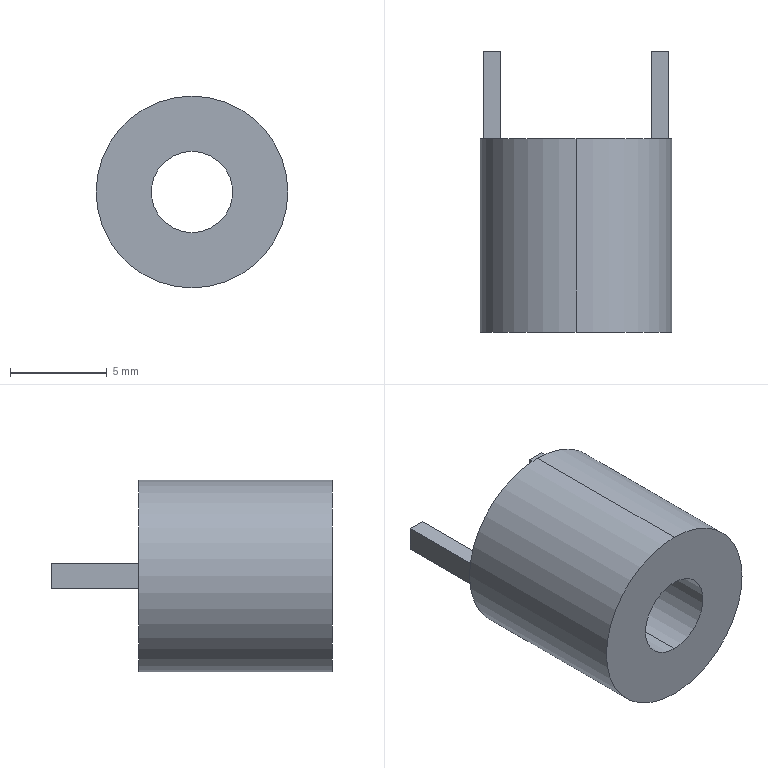Part | STEP file | 1 solid | 16 faces | box 9.9 x 14.5 x 9.9 mm | volume 641.755 mm3 | plane 12 | cylinder 4 | commonest cylinder face diameters 4.2 x2 9.9 x2
STEP:
#1=CARTESIAN_POINT('',(0.,0.,0.));
#2=DIRECTION('',(0.,0.,1.));
#3=DIRECTION('',(1.,0.,0.));
#4=AXIS2_PLACEMENT_3D('',#1,#2,#3);
#5=CARTESIAN_POINT('',(0.,0.,2.1));
#6=VERTEX_POINT('',#5);
#7=CARTESIAN_POINT('',(0.,10.,2.1));
#8=VERTEX_POINT('',#7);
#9=CARTESIAN_POINT('',(0.,10.,2.1));
#10=DIRECTION('',(0.,1.,0.));
#11=VECTOR('',#10,1.);
#12=LINE('',#9,#11);
#13=CARTESIAN_POINT('',(0.,10.,0.));
#14=DIRECTION('',(0.,1.,0.));
#15=DIRECTION('',(0.,0.,1.));
#16=AXIS2_PLACEMENT_3D('',#13,#14,#15);
#17=CYLINDRICAL_SURFACE('',#16,2.1);
#18=CARTESIAN_POINT('',(6.283,0.));
#19=DIRECTION('',(0.,1.));
#20=VECTOR('',#19,1.);
#21=LINE('',#18,#20);
#22=(GEOMETRIC_REPRESENTATION_CONTEXT(2)PARAMETRIC_REPRESENTATION_CONTEXT()REPRESENTATION_CONTEXT('',''));
#23=DEFINITIONAL_REPRESENTATION('',(#21),#22);
#24=PCURVE('',#17,#23);
#25=CARTESIAN_POINT('',(0.,10.,0.));
#26=DIRECTION('',(0.,1.,0.));
#27=DIRECTION('',(0.,0.,1.));
#28=AXIS2_PLACEMENT_3D('',#25,#26,#27);
#29=CYLINDRICAL_SURFACE('',#28,2.1);
#30=CARTESIAN_POINT('',(0.,0.));
#31=DIRECTION('',(0.,1.));
#32=VECTOR('',#31,1.);
#33=LINE('',#30,#32);
#34=(GEOMETRIC_REPRESENTATION_CONTEXT(2)PARAMETRIC_REPRESENTATION_CONTEXT()REPRESENTATION_CONTEXT('',''));
#35=DEFINITIONAL_REPRESENTATION('',(#33),#34);
#36=PCURVE('',#29,#35);
#37=SURFACE_CURVE('',#12,(#24,#36),.PCURVE_S1.);
#38=EDGE_CURVE('',#6,#8,#37,.T.);
#39=ORIENTED_EDGE('',*,*,#38,.T.);
#40=CARTESIAN_POINT('',(0.,10.,-2.1));
#41=VERTEX_POINT('',#40);
#42=CARTESIAN_POINT('',(0.,10.,0.));
#43=DIRECTION('',(0.,1.,0.));
#44=DIRECTION('',(0.,0.,1.));
#45=AXIS2_PLACEMENT_3D('',#42,#43,#44);
#46=CIRCLE('',#45,2.1);
#47=CARTESIAN_POINT('',(0.,0.));
#48=DIRECTION('',(1.,0.));
#49=VECTOR('',#48,1.);
#50=LINE('',#47,#49);
#51=(GEOMETRIC_REPRESENTATION_CONTEXT(2)PARAMETRIC_REPRESENTATION_CONTEXT()REPRESENTATION_CONTEXT('',''));
#52=DEFINITIONAL_REPRESENTATION('',(#50),#51);
#53=PCURVE('',#17,#52);
#54=CARTESIAN_POINT('',(0.,10.,0.));
#55=DIRECTION('',(0.,1.,0.));
#56=DIRECTION('',(0.,0.,1.));
#57=AXIS2_PLACEMENT_3D('',#54,#55,#56);
#58=PLANE('',#57);
#59=CARTESIAN_POINT('',(0.,0.));
#60=DIRECTION('',(1.,0.));
#61=AXIS2_PLACEMENT_2D('',#59,#60);
#62=CIRCLE('',#61,2.1);
#63=(GEOMETRIC_REPRESENTATION_CONTEXT(2)PARAMETRIC_REPRESENTATION_CONTEXT()REPRESENTATION_CONTEXT('',''));
#64=DEFINITIONAL_REPRESENTATION('',(#62),#63);
#65=PCURVE('',#58,#64);
#66=SURFACE_CURVE('',#46,(#53,#65),.PCURVE_S1.);
#67=EDGE_CURVE('',#41,#8,#66,.T.);
#68=ORIENTED_EDGE('',*,*,#67,.F.);
#69=CARTESIAN_POINT('',(0.,0.,-2.1));
#70=VERTEX_POINT('',#69);
#71=CARTESIAN_POINT('',(0.,10.,-2.1));
#72=DIRECTION('',(0.,1.,0.));
#73=VECTOR('',#72,1.);
#74=LINE('',#71,#73);
#75=CARTESIAN_POINT('',(3.142,0.));
#76=DIRECTION('',(0.,1.));
#77=VECTOR('',#76,1.);
#78=LINE('',#75,#77);
#79=(GEOMETRIC_REPRESENTATION_CONTEXT(2)PARAMETRIC_REPRESENTATION_CONTEXT()REPRESENTATION_CONTEXT('',''));
#80=DEFINITIONAL_REPRESENTATION('',(#78),#79);
#81=PCURVE('',#17,#80);
#82=CARTESIAN_POINT('',(3.142,0.));
#83=DIRECTION('',(0.,1.));
#84=VECTOR('',#83,1.);
#85=LINE('',#82,#84);
#86=(GEOMETRIC_REPRESENTATION_CONTEXT(2)PARAMETRIC_REPRESENTATION_CONTEXT()REPRESENTATION_CONTEXT('',''));
#87=DEFINITIONAL_REPRESENTATION('',(#85),#86);
#88=PCURVE('',#29,#87);
#89=SURFACE_CURVE('',#74,(#81,#88),.PCURVE_S1.);
#90=EDGE_CURVE('',#70,#41,#89,.T.);
#91=ORIENTED_EDGE('',*,*,#90,.F.);
#92=CARTESIAN_POINT('',(0.,0.,0.));
#93=DIRECTION('',(0.,1.,0.));
#94=DIRECTION('',(0.,0.,1.));
#95=AXIS2_PLACEMENT_3D('',#92,#93,#94);
#96=CIRCLE('',#95,2.1);
#97=CARTESIAN_POINT('',(0.,-10.));
#98=DIRECTION('',(1.,0.));
#99=VECTOR('',#98,1.);
#100=LINE('',#97,#99);
#101=(GEOMETRIC_REPRESENTATION_CONTEXT(2)PARAMETRIC_REPRESENTATION_CONTEXT()REPRESENTATION_CONTEXT('',''));
#102=DEFINITIONAL_REPRESENTATION('',(#100),#101);
#103=PCURVE('',#17,#102);
#104=CARTESIAN_POINT('',(0.,0.,0.));
#105=DIRECTION('',(0.,1.,0.));
#106=DIRECTION('',(0.,0.,1.));
#107=AXIS2_PLACEMENT_3D('',#104,#105,#106);
#108=PLANE('',#107);
#109=CARTESIAN_POINT('',(0.,0.));
#110=DIRECTION('',(1.,0.));
#111=AXIS2_PLACEMENT_2D('',#109,#110);
#112=CIRCLE('',#111,2.1);
#113=(GEOMETRIC_REPRESENTATION_CONTEXT(2)PARAMETRIC_REPRESENTATION_CONTEXT()REPRESENTATION_CONTEXT('',''));
#114=DEFINITIONAL_REPRESENTATION('',(#112),#113);
#115=PCURVE('',#108,#114);
#116=SURFACE_CURVE('',#96,(#103,#115),.PCURVE_S1.);
#117=EDGE_CURVE('',#70,#6,#116,.T.);
#118=ORIENTED_EDGE('',*,*,#117,.T.);
#119=EDGE_LOOP('',(#39,#68,#91,#118));
#120=FACE_BOUND('',#119,.F.);
#121=ADVANCED_FACE('',(#120),#17,.F.);
#122=CARTESIAN_POINT('',(0.,10.,4.95));
#123=VERTEX_POINT('',#122);
#124=CARTESIAN_POINT('',(0.,10.,-4.95));
#125=VERTEX_POINT('',#124);
#126=CARTESIAN_POINT('',(0.,10.,0.));
#127=DIRECTION('',(0.,1.,0.));
#128=DIRECTION('',(0.,0.,1.));
#129=AXIS2_PLACEMENT_3D('',#126,#127,#128);
#130=CIRCLE('',#129,4.95);
#131=CARTESIAN_POINT('',(0.,10.,0.));
#132=DIRECTION('',(0.,-1.,0.));
#133=DIRECTION('',(0.,0.,-1.));
#134=AXIS2_PLACEMENT_3D('',#131,#132,#133);
#135=CYLINDRICAL_SURFACE('',#134,4.95);
#136=CARTESIAN_POINT('',(3.142,0.));
#137=DIRECTION('',(-1.,0.));
#138=VECTOR('',#137,1.);
#139=LINE('',#136,#138);
#140=(GEOMETRIC_REPRESENTATION_CONTEXT(2)PARAMETRIC_REPRESENTATION_CONTEXT()REPRESENTATION_CONTEXT('',''));
#141=DEFINITIONAL_REPRESENTATION('',(#139),#140);
#142=PCURVE('',#135,#141);
#143=CARTESIAN_POINT('',(0.,0.));
#144=DIRECTION('',(1.,0.));
#145=AXIS2_PLACEMENT_2D('',#143,#144);
#146=CIRCLE('',#145,4.95);
#147=(GEOMETRIC_REPRESENTATION_CONTEXT(2)PARAMETRIC_REPRESENTATION_CONTEXT()REPRESENTATION_CONTEXT('',''));
#148=DEFINITIONAL_REPRESENTATION('',(#146),#147);
#149=PCURVE('',#58,#148);
#150=SURFACE_CURVE('',#130,(#142,#149),.PCURVE_S1.);
#151=EDGE_CURVE('',#123,#125,#150,.T.);
#152=ORIENTED_EDGE('',*,*,#151,.F.);
#153=CARTESIAN_POINT('',(0.,0.,4.95));
#154=VERTEX_POINT('',#153);
#155=CARTESIAN_POINT('',(0.,10.,4.95));
#156=DIRECTION('',(0.,-1.,0.));
#157=VECTOR('',#156,1.);
#158=LINE('',#155,#157);
#159=CARTESIAN_POINT('',(3.142,0.));
#160=DIRECTION('',(0.,1.));
#161=VECTOR('',#160,1.);
#162=LINE('',#159,#161);
#163=(GEOMETRIC_REPRESENTATION_CONTEXT(2)PARAMETRIC_REPRESENTATION_CONTEXT()REPRESENTATION_CONTEXT('',''));
#164=DEFINITIONAL_REPRESENTATION('',(#162),#163);
#165=PCURVE('',#135,#164);
#166=CARTESIAN_POINT('',(0.,10.,0.));
#167=DIRECTION('',(0.,-1.,0.));
#168=DIRECTION('',(0.,0.,-1.));
#169=AXIS2_PLACEMENT_3D('',#166,#167,#168);
#170=CYLINDRICAL_SURFACE('',#169,4.95);
#171=CARTESIAN_POINT('',(3.142,0.));
#172=DIRECTION('',(0.,1.));
#173=VECTOR('',#172,1.);
#174=LINE('',#171,#173);
#175=(GEOMETRIC_REPRESENTATION_CONTEXT(2)PARAMETRIC_REPRESENTATION_CONTEXT()REPRESENTATION_CONTEXT('',''));
#176=DEFINITIONAL_REPRESENTATION('',(#174),#175);
#177=PCURVE('',#170,#176);
#178=SURFACE_CURVE('',#158,(#165,#177),.PCURVE_S1.);
#179=EDGE_CURVE('',#123,#154,#178,.T.);
#180=ORIENTED_EDGE('',*,*,#179,.T.);
#181=CARTESIAN_POINT('',(0.,0.,-4.95));
#182=VERTEX_POINT('',#181);
#183=CARTESIAN_POINT('',(0.,0.,0.));
#184=DIRECTION('',(0.,1.,0.));
#185=DIRECTION('',(0.,0.,1.));
#186=AXIS2_PLACEMENT_3D('',#183,#184,#185);
#187=CIRCLE('',#186,4.95);
#188=CARTESIAN_POINT('',(3.142,10.));
#189=DIRECTION('',(-1.,0.));
#190=VECTOR('',#189,1.);
#191=LINE('',#188,#190);
#192=(GEOMETRIC_REPRESENTATION_CONTEXT(2)PARAMETRIC_REPRESENTATION_CONTEXT()REPRESENTATION_CONTEXT('',''));
#193=DEFINITIONAL_REPRESENTATION('',(#191),#192);
#194=PCURVE('',#135,#193);
#195=CARTESIAN_POINT('',(0.,0.));
#196=DIRECTION('',(1.,0.));
#197=AXIS2_PLACEMENT_2D('',#195,#196);
#198=CIRCLE('',#197,4.95);
#199=(GEOMETRIC_REPRESENTATION_CONTEXT(2)PARAMETRIC_REPRESENTATION_CONTEXT()REPRESENTATION_CONTEXT('',''));
#200=DEFINITIONAL_REPRESENTATION('',(#198),#199);
#201=PCURVE('',#108,#200);
#202=SURFACE_CURVE('',#187,(#194,#201),.PCURVE_S1.);
#203=EDGE_CURVE('',#154,#182,#202,.T.);
#204=ORIENTED_EDGE('',*,*,#203,.T.);
#205=CARTESIAN_POINT('',(0.,10.,-4.95));
#206=DIRECTION('',(0.,-1.,0.));
#207=VECTOR('',#206,1.);
#208=LINE('',#205,#207);
#209=CARTESIAN_POINT('',(0.,0.));
#210=DIRECTION('',(0.,1.));
#211=VECTOR('',#210,1.);
#212=LINE('',#209,#211);
#213=(GEOMETRIC_REPRESENTATION_CONTEXT(2)PARAMETRIC_REPRESENTATION_CONTEXT()REPRESENTATION_CONTEXT('',''));
#214=DEFINITIONAL_REPRESENTATION('',(#212),#213);
#215=PCURVE('',#135,#214);
#216=CARTESIAN_POINT('',(6.283,0.));
#217=DIRECTION('',(0.,1.));
#218=VECTOR('',#217,1.);
#219=LINE('',#216,#218);
#220=(GEOMETRIC_REPRESENTATION_CONTEXT(2)PARAMETRIC_REPRESENTATION_CONTEXT()REPRESENTATION_CONTEXT('',''));
#221=DEFINITIONAL_REPRESENTATION('',(#219),#220);
#222=PCURVE('',#170,#221);
#223=SURFACE_CURVE('',#208,(#215,#222),.PCURVE_S1.);
#224=EDGE_CURVE('',#125,#182,#223,.T.);
#225=ORIENTED_EDGE('',*,*,#224,.F.);
#226=EDGE_LOOP('',(#152,#180,#204,#225));
#227=FACE_BOUND('',#226,.T.);
#228=ADVANCED_FACE('',(#227),#135,.T.);
#229=ORIENTED_EDGE('',*,*,#179,.F.);
#230=CARTESIAN_POINT('',(0.,10.,0.));
#231=DIRECTION('',(0.,1.,0.));
#232=DIRECTION('',(0.,0.,1.));
#233=AXIS2_PLACEMENT_3D('',#230,#231,#232);
#234=CIRCLE('',#233,4.95);
#235=CARTESIAN_POINT('',(9.425,0.));
#236=DIRECTION('',(-1.,0.));
#237=VECTOR('',#236,1.);
#238=LINE('',#235,#237);
#239=(GEOMETRIC_REPRESENTATION_CONTEXT(2)PARAMETRIC_REPRESENTATION_CONTEXT()REPRESENTATION_CONTEXT('',''));
#240=DEFINITIONAL_REPRESENTATION('',(#238),#239);
#241=PCURVE('',#170,#240);
#242=CARTESIAN_POINT('',(0.,0.));
#243=DIRECTION('',(1.,0.));
#244=AXIS2_PLACEMENT_2D('',#242,#243);
#245=CIRCLE('',#244,4.95);
#246=(GEOMETRIC_REPRESENTATION_CONTEXT(2)PARAMETRIC_REPRESENTATION_CONTEXT()REPRESENTATION_CONTEXT('',''));
#247=DEFINITIONAL_REPRESENTATION('',(#245),#246);
#248=PCURVE('',#58,#247);
#249=SURFACE_CURVE('',#234,(#241,#248),.PCURVE_S1.);
#250=EDGE_CURVE('',#125,#123,#249,.T.);
#251=ORIENTED_EDGE('',*,*,#250,.F.);
#252=ORIENTED_EDGE('',*,*,#224,.T.);
#253=CARTESIAN_POINT('',(0.,0.,0.));
#254=DIRECTION('',(0.,1.,0.));
#255=DIRECTION('',(0.,0.,1.));
#256=AXIS2_PLACEMENT_3D('',#253,#254,#255);
#257=CIRCLE('',#256,4.95);
#258=CARTESIAN_POINT('',(9.425,10.));
#259=DIRECTION('',(-1.,0.));
#260=VECTOR('',#259,1.);
#261=LINE('',#258,#260);
#262=(GEOMETRIC_REPRESENTATION_CONTEXT(2)PARAMETRIC_REPRESENTATION_CONTEXT()REPRESENTATION_CONTEXT('',''));
#263=DEFINITIONAL_REPRESENTATION('',(#261),#262);
#264=PCURVE('',#170,#263);
#265=CARTESIAN_POINT('',(0.,0.));
#266=DIRECTION('',(1.,0.));
#267=AXIS2_PLACEMENT_2D('',#265,#266);
#268=CIRCLE('',#267,4.95);
#269=(GEOMETRIC_REPRESENTATION_CONTEXT(2)PARAMETRIC_REPRESENTATION_CONTEXT()REPRESENTATION_CONTEXT('',''));
#270=DEFINITIONAL_REPRESENTATION('',(#268),#269);
#271=PCURVE('',#108,#270);
#272=SURFACE_CURVE('',#257,(#264,#271),.PCURVE_S1.);
#273=EDGE_CURVE('',#182,#154,#272,.T.);
#274=ORIENTED_EDGE('',*,*,#273,.T.);
#275=EDGE_LOOP('',(#229,#251,#252,#274));
#276=FACE_BOUND('',#275,.T.);
#277=ADVANCED_FACE('',(#276),#170,.T.);
#278=CARTESIAN_POINT('',(4.8,10.,-0.65));
#279=VERTEX_POINT('',#278);
#280=CARTESIAN_POINT('',(3.9,10.,-0.65));
#281=VERTEX_POINT('',#280);
#282=CARTESIAN_POINT('',(4.907,10.,-0.65));
#283=DIRECTION('',(-1.,0.,0.));
#284=VECTOR('',#283,1.);
#285=LINE('',#282,#284);
#286=CARTESIAN_POINT('',(-0.65,4.907));
#287=DIRECTION('',(0.,-1.));
#288=VECTOR('',#287,1.);
#289=LINE('',#286,#288);
#290=(GEOMETRIC_REPRESENTATION_CONTEXT(2)PARAMETRIC_REPRESENTATION_CONTEXT()REPRESENTATION_CONTEXT('',''));
#291=DEFINITIONAL_REPRESENTATION('',(#289),#290);
#292=PCURVE('',#58,#291);
#293=CARTESIAN_POINT('',(4.907,14.5,-0.65));
#294=DIRECTION('',(0.,0.,1.));
#295=DIRECTION('',(1.,0.,0.));
#296=AXIS2_PLACEMENT_3D('',#293,#294,#295);
#297=PLANE('',#296);
#298=CARTESIAN_POINT('',(0.,-4.5));
#299=DIRECTION('',(-1.,0.));
#300=VECTOR('',#299,1.);
#301=LINE('',#298,#300);
#302=(GEOMETRIC_REPRESENTATION_CONTEXT(2)PARAMETRIC_REPRESENTATION_CONTEXT()REPRESENTATION_CONTEXT('',''));
#303=DEFINITIONAL_REPRESENTATION('',(#301),#302);
#304=PCURVE('',#297,#303);
#305=SURFACE_CURVE('',#285,(#292,#304),.PCURVE_S1.);
#306=EDGE_CURVE('',#279,#281,#305,.T.);
#307=ORIENTED_EDGE('',*,*,#306,.F.);
#308=CARTESIAN_POINT('',(4.8,10.,0.65));
#309=VERTEX_POINT('',#308);
#310=CARTESIAN_POINT('',(4.8,10.,-0.65));
#311=DIRECTION('',(0.,0.,-1.));
#312=VECTOR('',#311,1.);
#313=LINE('',#310,#312);
#314=CARTESIAN_POINT('',(-0.65,4.8));
#315=DIRECTION('',(-1.,0.));
#316=VECTOR('',#315,1.);
#317=LINE('',#314,#316);
#318=(GEOMETRIC_REPRESENTATION_CONTEXT(2)PARAMETRIC_REPRESENTATION_CONTEXT()REPRESENTATION_CONTEXT('',''));
#319=DEFINITIONAL_REPRESENTATION('',(#317),#318);
#320=PCURVE('',#58,#319);
#321=CARTESIAN_POINT('',(4.8,8.691,-0.65));
#322=DIRECTION('',(-1.,0.,0.));
#323=DIRECTION('',(0.,0.,1.));
#324=AXIS2_PLACEMENT_3D('',#321,#322,#323);
#325=PLANE('',#324);
#326=CARTESIAN_POINT('',(0.,1.309));
#327=DIRECTION('',(-1.,0.));
#328=VECTOR('',#327,1.);
#329=LINE('',#326,#328);
#330=(GEOMETRIC_REPRESENTATION_CONTEXT(2)PARAMETRIC_REPRESENTATION_CONTEXT()REPRESENTATION_CONTEXT('',''));
#331=DEFINITIONAL_REPRESENTATION('',(#329),#330);
#332=PCURVE('',#325,#331);
#333=SURFACE_CURVE('',#313,(#320,#332),.PCURVE_S1.);
#334=EDGE_CURVE('',#309,#279,#333,.T.);
#335=ORIENTED_EDGE('',*,*,#334,.F.);
#336=CARTESIAN_POINT('',(3.9,10.,0.65));
#337=VERTEX_POINT('',#336);
#338=CARTESIAN_POINT('',(3.9,10.,0.65));
#339=DIRECTION('',(1.,0.,0.));
#340=VECTOR('',#339,1.);
#341=LINE('',#338,#340);
#342=CARTESIAN_POINT('',(0.65,3.9));
#343=DIRECTION('',(0.,1.));
#344=VECTOR('',#343,1.);
#345=LINE('',#342,#344);
#346=(GEOMETRIC_REPRESENTATION_CONTEXT(2)PARAMETRIC_REPRESENTATION_CONTEXT()REPRESENTATION_CONTEXT('',''));
#347=DEFINITIONAL_REPRESENTATION('',(#345),#346);
#348=PCURVE('',#58,#347);
#349=CARTESIAN_POINT('',(3.9,14.5,0.65));
#350=DIRECTION('',(0.,0.,-1.));
#351=DIRECTION('',(-1.,0.,0.));
#352=AXIS2_PLACEMENT_3D('',#349,#350,#351);
#353=PLANE('',#352);
#354=CARTESIAN_POINT('',(0.,-4.5));
#355=DIRECTION('',(-1.,0.));
#356=VECTOR('',#355,1.);
#357=LINE('',#354,#356);
#358=(GEOMETRIC_REPRESENTATION_CONTEXT(2)PARAMETRIC_REPRESENTATION_CONTEXT()REPRESENTATION_CONTEXT('',''));
#359=DEFINITIONAL_REPRESENTATION('',(#357),#358);
#360=PCURVE('',#353,#359);
#361=SURFACE_CURVE('',#341,(#348,#360),.PCURVE_S1.);
#362=EDGE_CURVE('',#337,#309,#361,.T.);
#363=ORIENTED_EDGE('',*,*,#362,.F.);
#364=CARTESIAN_POINT('',(3.9,10.,-0.65));
#365=DIRECTION('',(0.,0.,1.));
#366=VECTOR('',#365,1.);
#367=LINE('',#364,#366);
#368=CARTESIAN_POINT('',(-0.65,3.9));
#369=DIRECTION('',(1.,0.));
#370=VECTOR('',#369,1.);
#371=LINE('',#368,#370);
#372=(GEOMETRIC_REPRESENTATION_CONTEXT(2)PARAMETRIC_REPRESENTATION_CONTEXT()REPRESENTATION_CONTEXT('',''));
#373=DEFINITIONAL_REPRESENTATION('',(#371),#372);
#374=PCURVE('',#58,#373);
#375=CARTESIAN_POINT('',(3.9,14.5,-0.65));
#376=DIRECTION('',(1.,0.,0.));
#377=DIRECTION('',(0.,0.,-1.));
#378=AXIS2_PLACEMENT_3D('',#375,#376,#377);
#379=PLANE('',#378);
#380=CARTESIAN_POINT('',(0.,-4.5));
#381=DIRECTION('',(-1.,0.));
#382=VECTOR('',#381,1.);
#383=LINE('',#380,#382);
#384=(GEOMETRIC_REPRESENTATION_CONTEXT(2)PARAMETRIC_REPRESENTATION_CONTEXT()REPRESENTATION_CONTEXT('',''));
#385=DEFINITIONAL_REPRESENTATION('',(#383),#384);
#386=PCURVE('',#379,#385);
#387=SURFACE_CURVE('',#367,(#374,#386),.PCURVE_S1.);
#388=EDGE_CURVE('',#281,#337,#387,.T.);
#389=ORIENTED_EDGE('',*,*,#388,.F.);
#390=EDGE_LOOP('',(#307,#335,#363,#389));
#391=FACE_BOUND('',#390,.T.);
#392=CARTESIAN_POINT('',(-4.8,10.,-0.65));
#393=VERTEX_POINT('',#392);
#394=CARTESIAN_POINT('',(-4.8,10.,0.65));
#395=VERTEX_POINT('',#394);
#396=CARTESIAN_POINT('',(-4.8,10.,-0.65));
#397=DIRECTION('',(0.,0.,1.));
#398=VECTOR('',#397,1.);
#399=LINE('',#396,#398);
#400=CARTESIAN_POINT('',(-0.65,-4.8));
#401=DIRECTION('',(1.,0.));
#402=VECTOR('',#401,1.);
#403=LINE('',#400,#402);
#404=(GEOMETRIC_REPRESENTATION_CONTEXT(2)PARAMETRIC_REPRESENTATION_CONTEXT()REPRESENTATION_CONTEXT('',''));
#405=DEFINITIONAL_REPRESENTATION('',(#403),#404);
#406=PCURVE('',#58,#405);
#407=CARTESIAN_POINT('',(-4.8,8.691,-0.65));
#408=DIRECTION('',(1.,0.,0.));
#409=DIRECTION('',(0.,0.,-1.));
#410=AXIS2_PLACEMENT_3D('',#407,#408,#409);
#411=PLANE('',#410);
#412=CARTESIAN_POINT('',(0.,1.309));
#413=DIRECTION('',(-1.,0.));
#414=VECTOR('',#413,1.);
#415=LINE('',#412,#414);
#416=(GEOMETRIC_REPRESENTATION_CONTEXT(2)PARAMETRIC_REPRESENTATION_CONTEXT()REPRESENTATION_CONTEXT('',''));
#417=DEFINITIONAL_REPRESENTATION('',(#415),#416);
#418=PCURVE('',#411,#417);
#419=SURFACE_CURVE('',#399,(#406,#418),.PCURVE_S1.);
#420=EDGE_CURVE('',#393,#395,#419,.T.);
#421=ORIENTED_EDGE('',*,*,#420,.F.);
#422=CARTESIAN_POINT('',(-3.9,10.,-0.65));
#423=VERTEX_POINT('',#422);
#424=CARTESIAN_POINT('',(-4.907,10.,-0.65));
#425=DIRECTION('',(-1.,0.,0.));
#426=VECTOR('',#425,1.);
#427=LINE('',#424,#426);
#428=CARTESIAN_POINT('',(-0.65,-4.907));
#429=DIRECTION('',(0.,-1.));
#430=VECTOR('',#429,1.);
#431=LINE('',#428,#430);
#432=(GEOMETRIC_REPRESENTATION_CONTEXT(2)PARAMETRIC_REPRESENTATION_CONTEXT()REPRESENTATION_CONTEXT('',''));
#433=DEFINITIONAL_REPRESENTATION('',(#431),#432);
#434=PCURVE('',#58,#433);
#435=CARTESIAN_POINT('',(-4.907,14.5,-0.65));
#436=DIRECTION('',(0.,0.,1.));
#437=DIRECTION('',(1.,0.,0.));
#438=AXIS2_PLACEMENT_3D('',#435,#436,#437);
#439=PLANE('',#438);
#440=CARTESIAN_POINT('',(0.,-4.5));
#441=DIRECTION('',(-1.,0.));
#442=VECTOR('',#441,1.);
#443=LINE('',#440,#442);
#444=(GEOMETRIC_REPRESENTATION_CONTEXT(2)PARAMETRIC_REPRESENTATION_CONTEXT()REPRESENTATION_CONTEXT('',''));
#445=DEFINITIONAL_REPRESENTATION('',(#443),#444);
#446=PCURVE('',#439,#445);
#447=SURFACE_CURVE('',#427,(#434,#446),.PCURVE_S1.);
#448=EDGE_CURVE('',#423,#393,#447,.T.);
#449=ORIENTED_EDGE('',*,*,#448,.F.);
#450=CARTESIAN_POINT('',(-3.9,10.,0.65));
#451=VERTEX_POINT('',#450);
#452=CARTESIAN_POINT('',(-3.9,10.,-0.65));
#453=DIRECTION('',(0.,0.,-1.));
#454=VECTOR('',#453,1.);
#455=LINE('',#452,#454);
#456=CARTESIAN_POINT('',(-0.65,-3.9));
#457=DIRECTION('',(-1.,0.));
#458=VECTOR('',#457,1.);
#459=LINE('',#456,#458);
#460=(GEOMETRIC_REPRESENTATION_CONTEXT(2)PARAMETRIC_REPRESENTATION_CONTEXT()REPRESENTATION_CONTEXT('',''));
#461=DEFINITIONAL_REPRESENTATION('',(#459),#460);
#462=PCURVE('',#58,#461);
#463=CARTESIAN_POINT('',(-3.9,14.5,-0.65));
#464=DIRECTION('',(-1.,0.,0.));
#465=DIRECTION('',(0.,0.,1.));
#466=AXIS2_PLACEMENT_3D('',#463,#464,#465);
#467=PLANE('',#466);
#468=CARTESIAN_POINT('',(0.,-4.5));
#469=DIRECTION('',(-1.,0.));
#470=VECTOR('',#469,1.);
#471=LINE('',#468,#470);
#472=(GEOMETRIC_REPRESENTATION_CONTEXT(2)PARAMETRIC_REPRESENTATION_CONTEXT()REPRESENTATION_CONTEXT('',''));
#473=DEFINITIONAL_REPRESENTATION('',(#471),#472);
#474=PCURVE('',#467,#473);
#475=SURFACE_CURVE('',#455,(#462,#474),.PCURVE_S1.);
#476=EDGE_CURVE('',#451,#423,#475,.T.);
#477=ORIENTED_EDGE('',*,*,#476,.F.);
#478=CARTESIAN_POINT('',(-3.9,10.,0.65));
#479=DIRECTION('',(1.,0.,0.));
#480=VECTOR('',#479,1.);
#481=LINE('',#478,#480);
#482=CARTESIAN_POINT('',(0.65,-3.9));
#483=DIRECTION('',(0.,1.));
#484=VECTOR('',#483,1.);
#485=LINE('',#482,#484);
#486=(GEOMETRIC_REPRESENTATION_CONTEXT(2)PARAMETRIC_REPRESENTATION_CONTEXT()REPRESENTATION_CONTEXT('',''));
#487=DEFINITIONAL_REPRESENTATION('',(#485),#486);
#488=PCURVE('',#58,#487);
#489=CARTESIAN_POINT('',(-3.9,14.5,0.65));
#490=DIRECTION('',(0.,0.,-1.));
#491=DIRECTION('',(-1.,0.,0.));
#492=AXIS2_PLACEMENT_3D('',#489,#490,#491);
#493=PLANE('',#492);
#494=CARTESIAN_POINT('',(0.,-4.5));
#495=DIRECTION('',(-1.,0.));
#496=VECTOR('',#495,1.);
#497=LINE('',#494,#496);
#498=(GEOMETRIC_REPRESENTATION_CONTEXT(2)PARAMETRIC_REPRESENTATION_CONTEXT()REPRESENTATION_CONTEXT('',''));
#499=DEFINITIONAL_REPRESENTATION('',(#497),#498);
#500=PCURVE('',#493,#499);
#501=SURFACE_CURVE('',#481,(#488,#500),.PCURVE_S1.);
#502=EDGE_CURVE('',#395,#451,#501,.T.);
#503=ORIENTED_EDGE('',*,*,#502,.F.);
#504=EDGE_LOOP('',(#421,#449,#477,#503));
#505=FACE_BOUND('',#504,.T.);
#506=CARTESIAN_POINT('',(0.,10.,0.));
#507=DIRECTION('',(0.,1.,0.));
#508=DIRECTION('',(0.,0.,1.));
#509=AXIS2_PLACEMENT_3D('',#506,#507,#508);
#510=CIRCLE('',#509,2.1);
#511=CARTESIAN_POINT('',(0.,0.));
#512=DIRECTION('',(1.,0.));
#513=AXIS2_PLACEMENT_2D('',#511,#512);
#514=CIRCLE('',#513,2.1);
#515=(GEOMETRIC_REPRESENTATION_CONTEXT(2)PARAMETRIC_REPRESENTATION_CONTEXT()REPRESENTATION_CONTEXT('',''));
#516=DEFINITIONAL_REPRESENTATION('',(#514),#515);
#517=PCURVE('',#58,#516);
#518=CARTESIAN_POINT('',(0.,0.));
#519=DIRECTION('',(1.,0.));
#520=VECTOR('',#519,1.);
#521=LINE('',#518,#520);
#522=(GEOMETRIC_REPRESENTATION_CONTEXT(2)PARAMETRIC_REPRESENTATION_CONTEXT()REPRESENTATION_CONTEXT('',''));
#523=DEFINITIONAL_REPRESENTATION('',(#521),#522);
#524=PCURVE('',#29,#523);
#525=SURFACE_CURVE('',#510,(#517,#524),.PCURVE_S1.);
#526=EDGE_CURVE('',#8,#41,#525,.T.);
#527=ORIENTED_EDGE('',*,*,#526,.F.);
#528=ORIENTED_EDGE('',*,*,#67,.F.);
#529=EDGE_LOOP('',(#527,#528));
#530=FACE_BOUND('',#529,.T.);
#531=ORIENTED_EDGE('',*,*,#250,.T.);
#532=ORIENTED_EDGE('',*,*,#151,.T.);
#533=EDGE_LOOP('',(#531,#532));
#534=FACE_BOUND('',#533,.T.);
#535=ADVANCED_FACE('',(#391,#505,#530,#534),#58,.T.);
#536=CARTESIAN_POINT('',(0.,0.,0.));
#537=DIRECTION('',(0.,1.,0.));
#538=DIRECTION('',(0.,0.,1.));
#539=AXIS2_PLACEMENT_3D('',#536,#537,#538);
#540=CIRCLE('',#539,2.1);
#541=CARTESIAN_POINT('',(0.,0.));
#542=DIRECTION('',(1.,0.));
#543=AXIS2_PLACEMENT_2D('',#541,#542);
#544=CIRCLE('',#543,2.1);
#545=(GEOMETRIC_REPRESENTATION_CONTEXT(2)PARAMETRIC_REPRESENTATION_CONTEXT()REPRESENTATION_CONTEXT('',''));
#546=DEFINITIONAL_REPRESENTATION('',(#544),#545);
#547=PCURVE('',#108,#546);
#548=CARTESIAN_POINT('',(0.,-10.));
#549=DIRECTION('',(1.,0.));
#550=VECTOR('',#549,1.);
#551=LINE('',#548,#550);
#552=(GEOMETRIC_REPRESENTATION_CONTEXT(2)PARAMETRIC_REPRESENTATION_CONTEXT()REPRESENTATION_CONTEXT('',''));
#553=DEFINITIONAL_REPRESENTATION('',(#551),#552);
#554=PCURVE('',#29,#553);
#555=SURFACE_CURVE('',#540,(#547,#554),.PCURVE_S1.);
#556=EDGE_CURVE('',#6,#70,#555,.T.);
#557=ORIENTED_EDGE('',*,*,#556,.T.);
#558=ORIENTED_EDGE('',*,*,#117,.T.);
#559=EDGE_LOOP('',(#557,#558));
#560=FACE_BOUND('',#559,.T.);
#561=ORIENTED_EDGE('',*,*,#273,.F.);
#562=ORIENTED_EDGE('',*,*,#203,.F.);
#563=EDGE_LOOP('',(#561,#562));
#564=FACE_BOUND('',#563,.T.);
#565=ADVANCED_FACE('',(#560,#564),#108,.F.);
#566=ORIENTED_EDGE('',*,*,#526,.F.);
#567=ORIENTED_EDGE('',*,*,#38,.F.);
#568=ORIENTED_EDGE('',*,*,#556,.T.);
#569=ORIENTED_EDGE('',*,*,#90,.T.);
#570=EDGE_LOOP('',(#566,#567,#568,#569));
#571=FACE_BOUND('',#570,.F.);
#572=ADVANCED_FACE('',(#571),#29,.F.);
#573=CARTESIAN_POINT('',(4.8,14.5,-0.65));
#574=VERTEX_POINT('',#573);
#575=CARTESIAN_POINT('',(3.9,14.5,-0.65));
#576=VERTEX_POINT('',#575);
#577=CARTESIAN_POINT('',(4.907,14.5,-0.65));
#578=DIRECTION('',(-1.,0.,0.));
#579=VECTOR('',#578,1.);
#580=LINE('',#577,#579);
#581=CARTESIAN_POINT('',(0.,0.));
#582=DIRECTION('',(-1.,0.));
#583=VECTOR('',#582,1.);
#584=LINE('',#581,#583);
#585=(GEOMETRIC_REPRESENTATION_CONTEXT(2)PARAMETRIC_REPRESENTATION_CONTEXT()REPRESENTATION_CONTEXT('',''));
#586=DEFINITIONAL_REPRESENTATION('',(#584),#585);
#587=PCURVE('',#297,#586);
#588=CARTESIAN_POINT('',(0.,14.5,0.));
#589=DIRECTION('',(0.,1.,0.));
#590=DIRECTION('',(0.,0.,1.));
#591=AXIS2_PLACEMENT_3D('',#588,#589,#590);
#592=PLANE('',#591);
#593=CARTESIAN_POINT('',(-0.65,4.907));
#594=DIRECTION('',(0.,-1.));
#595=VECTOR('',#594,1.);
#596=LINE('',#593,#595);
#597=(GEOMETRIC_REPRESENTATION_CONTEXT(2)PARAMETRIC_REPRESENTATION_CONTEXT()REPRESENTATION_CONTEXT('',''));
#598=DEFINITIONAL_REPRESENTATION('',(#596),#597);
#599=PCURVE('',#592,#598);
#600=SURFACE_CURVE('',#580,(#587,#599),.PCURVE_S1.);
#601=EDGE_CURVE('',#574,#576,#600,.T.);
#602=ORIENTED_EDGE('',*,*,#601,.F.);
#603=CARTESIAN_POINT('',(4.8,8.691,-0.65));
#604=DIRECTION('',(0.,1.,0.));
#605=VECTOR('',#604,1.);
#606=LINE('',#603,#605);
#607=CARTESIAN_POINT('',(-0.1071,-5.809));
#608=DIRECTION('',(0.,1.));
#609=VECTOR('',#608,1.);
#610=LINE('',#607,#609);
#611=(GEOMETRIC_REPRESENTATION_CONTEXT(2)PARAMETRIC_REPRESENTATION_CONTEXT()REPRESENTATION_CONTEXT('',''));
#612=DEFINITIONAL_REPRESENTATION('',(#610),#611);
#613=PCURVE('',#297,#612);
#614=CARTESIAN_POINT('',(0.,0.));
#615=DIRECTION('',(0.,1.));
#616=VECTOR('',#615,1.);
#617=LINE('',#614,#616);
#618=(GEOMETRIC_REPRESENTATION_CONTEXT(2)PARAMETRIC_REPRESENTATION_CONTEXT()REPRESENTATION_CONTEXT('',''));
#619=DEFINITIONAL_REPRESENTATION('',(#617),#618);
#620=PCURVE('',#325,#619);
#621=SURFACE_CURVE('',#606,(#613,#620),.PCURVE_S1.);
#622=EDGE_CURVE('',#279,#574,#621,.T.);
#623=ORIENTED_EDGE('',*,*,#622,.F.);
#624=ORIENTED_EDGE('',*,*,#306,.T.);
#625=CARTESIAN_POINT('',(3.9,14.5,-0.65));
#626=DIRECTION('',(0.,-1.,0.));
#627=VECTOR('',#626,1.);
#628=LINE('',#625,#627);
#629=CARTESIAN_POINT('',(-1.007,0.));
#630=DIRECTION('',(0.,-1.));
#631=VECTOR('',#630,1.);
#632=LINE('',#629,#631);
#633=(GEOMETRIC_REPRESENTATION_CONTEXT(2)PARAMETRIC_REPRESENTATION_CONTEXT()REPRESENTATION_CONTEXT('',''));
#634=DEFINITIONAL_REPRESENTATION('',(#632),#633);
#635=PCURVE('',#297,#634);
#636=CARTESIAN_POINT('',(0.,0.));
#637=DIRECTION('',(0.,-1.));
#638=VECTOR('',#637,1.);
#639=LINE('',#636,#638);
#640=(GEOMETRIC_REPRESENTATION_CONTEXT(2)PARAMETRIC_REPRESENTATION_CONTEXT()REPRESENTATION_CONTEXT('',''));
#641=DEFINITIONAL_REPRESENTATION('',(#639),#640);
#642=PCURVE('',#379,#641);
#643=SURFACE_CURVE('',#628,(#635,#642),.PCURVE_S1.);
#644=EDGE_CURVE('',#576,#281,#643,.T.);
#645=ORIENTED_EDGE('',*,*,#644,.F.);
#646=EDGE_LOOP('',(#602,#623,#624,#645));
#647=FACE_BOUND('',#646,.T.);
#648=ADVANCED_FACE('',(#647),#297,.F.);
#649=ORIENTED_EDGE('',*,*,#388,.T.);
#650=CARTESIAN_POINT('',(3.9,14.5,0.65));
#651=VERTEX_POINT('',#650);
#652=CARTESIAN_POINT('',(3.9,14.5,0.65));
#653=DIRECTION('',(0.,-1.,0.));
#654=VECTOR('',#653,1.);
#655=LINE('',#652,#654);
#656=CARTESIAN_POINT('',(-1.3,0.));
#657=DIRECTION('',(0.,-1.));
#658=VECTOR('',#657,1.);
#659=LINE('',#656,#658);
#660=(GEOMETRIC_REPRESENTATION_CONTEXT(2)PARAMETRIC_REPRESENTATION_CONTEXT()REPRESENTATION_CONTEXT('',''));
#661=DEFINITIONAL_REPRESENTATION('',(#659),#660);
#662=PCURVE('',#379,#661);
#663=CARTESIAN_POINT('',(0.,0.));
#664=DIRECTION('',(0.,-1.));
#665=VECTOR('',#664,1.);
#666=LINE('',#663,#665);
#667=(GEOMETRIC_REPRESENTATION_CONTEXT(2)PARAMETRIC_REPRESENTATION_CONTEXT()REPRESENTATION_CONTEXT('',''));
#668=DEFINITIONAL_REPRESENTATION('',(#666),#667);
#669=PCURVE('',#353,#668);
#670=SURFACE_CURVE('',#655,(#662,#669),.PCURVE_S1.);
#671=EDGE_CURVE('',#651,#337,#670,.T.);
#672=ORIENTED_EDGE('',*,*,#671,.F.);
#673=CARTESIAN_POINT('',(3.9,14.5,-0.65));
#674=DIRECTION('',(0.,0.,1.));
#675=VECTOR('',#674,1.);
#676=LINE('',#673,#675);
#677=CARTESIAN_POINT('',(0.,0.));
#678=DIRECTION('',(-1.,0.));
#679=VECTOR('',#678,1.);
#680=LINE('',#677,#679);
#681=(GEOMETRIC_REPRESENTATION_CONTEXT(2)PARAMETRIC_REPRESENTATION_CONTEXT()REPRESENTATION_CONTEXT('',''));
#682=DEFINITIONAL_REPRESENTATION('',(#680),#681);
#683=PCURVE('',#379,#682);
#684=CARTESIAN_POINT('',(-0.65,3.9));
#685=DIRECTION('',(1.,0.));
#686=VECTOR('',#685,1.);
#687=LINE('',#684,#686);
#688=(GEOMETRIC_REPRESENTATION_CONTEXT(2)PARAMETRIC_REPRESENTATION_CONTEXT()REPRESENTATION_CONTEXT('',''));
#689=DEFINITIONAL_REPRESENTATION('',(#687),#688);
#690=PCURVE('',#592,#689);
#691=SURFACE_CURVE('',#676,(#683,#690),.PCURVE_S1.);
#692=EDGE_CURVE('',#576,#651,#691,.T.);
#693=ORIENTED_EDGE('',*,*,#692,.F.);
#694=ORIENTED_EDGE('',*,*,#644,.T.);
#695=EDGE_LOOP('',(#649,#672,#693,#694));
#696=FACE_BOUND('',#695,.T.);
#697=ADVANCED_FACE('',(#696),#379,.F.);
#698=ORIENTED_EDGE('',*,*,#362,.T.);
#699=CARTESIAN_POINT('',(4.8,14.5,0.65));
#700=VERTEX_POINT('',#699);
#701=CARTESIAN_POINT('',(4.8,8.691,0.65));
#702=DIRECTION('',(0.,1.,0.));
#703=VECTOR('',#702,1.);
#704=LINE('',#701,#703);
#705=CARTESIAN_POINT('',(-0.9,-5.809));
#706=DIRECTION('',(0.,1.));
#707=VECTOR('',#706,1.);
#708=LINE('',#705,#707);
#709=(GEOMETRIC_REPRESENTATION_CONTEXT(2)PARAMETRIC_REPRESENTATION_CONTEXT()REPRESENTATION_CONTEXT('',''));
#710=DEFINITIONAL_REPRESENTATION('',(#708),#709);
#711=PCURVE('',#353,#710);
#712=CARTESIAN_POINT('',(1.3,0.));
#713=DIRECTION('',(0.,1.));
#714=VECTOR('',#713,1.);
#715=LINE('',#712,#714);
#716=(GEOMETRIC_REPRESENTATION_CONTEXT(2)PARAMETRIC_REPRESENTATION_CONTEXT()REPRESENTATION_CONTEXT('',''));
#717=DEFINITIONAL_REPRESENTATION('',(#715),#716);
#718=PCURVE('',#325,#717);
#719=SURFACE_CURVE('',#704,(#711,#718),.PCURVE_S1.);
#720=EDGE_CURVE('',#309,#700,#719,.T.);
#721=ORIENTED_EDGE('',*,*,#720,.T.);
#722=CARTESIAN_POINT('',(3.9,14.5,0.65));
#723=DIRECTION('',(1.,0.,0.));
#724=VECTOR('',#723,1.);
#725=LINE('',#722,#724);
#726=CARTESIAN_POINT('',(0.,0.));
#727=DIRECTION('',(-1.,0.));
#728=VECTOR('',#727,1.);
#729=LINE('',#726,#728);
#730=(GEOMETRIC_REPRESENTATION_CONTEXT(2)PARAMETRIC_REPRESENTATION_CONTEXT()REPRESENTATION_CONTEXT('',''));
#731=DEFINITIONAL_REPRESENTATION('',(#729),#730);
#732=PCURVE('',#353,#731);
#733=CARTESIAN_POINT('',(0.65,3.9));
#734=DIRECTION('',(0.,1.));
#735=VECTOR('',#734,1.);
#736=LINE('',#733,#735);
#737=(GEOMETRIC_REPRESENTATION_CONTEXT(2)PARAMETRIC_REPRESENTATION_CONTEXT()REPRESENTATION_CONTEXT('',''));
#738=DEFINITIONAL_REPRESENTATION('',(#736),#737);
#739=PCURVE('',#592,#738);
#740=SURFACE_CURVE('',#725,(#732,#739),.PCURVE_S1.);
#741=EDGE_CURVE('',#651,#700,#740,.T.);
#742=ORIENTED_EDGE('',*,*,#741,.F.);
#743=ORIENTED_EDGE('',*,*,#671,.T.);
#744=EDGE_LOOP('',(#698,#721,#742,#743));
#745=FACE_BOUND('',#744,.T.);
#746=ADVANCED_FACE('',(#745),#353,.F.);
#747=CARTESIAN_POINT('',(4.8,14.5,-0.65));
#748=DIRECTION('',(0.,0.,1.));
#749=VECTOR('',#748,1.);
#750=LINE('',#747,#749);
#751=CARTESIAN_POINT('',(-0.65,4.8));
#752=DIRECTION('',(1.,0.));
#753=VECTOR('',#752,1.);
#754=LINE('',#751,#753);
#755=(GEOMETRIC_REPRESENTATION_CONTEXT(2)PARAMETRIC_REPRESENTATION_CONTEXT()REPRESENTATION_CONTEXT('',''));
#756=DEFINITIONAL_REPRESENTATION('',(#754),#755);
#757=PCURVE('',#592,#756);
#758=CARTESIAN_POINT('',(0.,5.809));
#759=DIRECTION('',(1.,0.));
#760=VECTOR('',#759,1.);
#761=LINE('',#758,#760);
#762=(GEOMETRIC_REPRESENTATION_CONTEXT(2)PARAMETRIC_REPRESENTATION_CONTEXT()REPRESENTATION_CONTEXT('',''));
#763=DEFINITIONAL_REPRESENTATION('',(#761),#762);
#764=PCURVE('',#325,#763);
#765=SURFACE_CURVE('',#750,(#757,#764),.PCURVE_S1.);
#766=EDGE_CURVE('',#574,#700,#765,.T.);
#767=ORIENTED_EDGE('',*,*,#766,.F.);
#768=ORIENTED_EDGE('',*,*,#601,.T.);
#769=ORIENTED_EDGE('',*,*,#692,.T.);
#770=ORIENTED_EDGE('',*,*,#741,.T.);
#771=EDGE_LOOP('',(#767,#768,#769,#770));
#772=FACE_BOUND('',#771,.T.);
#773=ADVANCED_FACE('',(#772),#592,.T.);
#774=ORIENTED_EDGE('',*,*,#476,.T.);
#775=CARTESIAN_POINT('',(-3.9,14.5,-0.65));
#776=VERTEX_POINT('',#775);
#777=CARTESIAN_POINT('',(-3.9,14.5,-0.65));
#778=DIRECTION('',(0.,-1.,0.));
#779=VECTOR('',#778,1.);
#780=LINE('',#777,#779);
#781=CARTESIAN_POINT('',(0.,0.));
#782=DIRECTION('',(0.,-1.));
#783=VECTOR('',#782,1.);
#784=LINE('',#781,#783);
#785=(GEOMETRIC_REPRESENTATION_CONTEXT(2)PARAMETRIC_REPRESENTATION_CONTEXT()REPRESENTATION_CONTEXT('',''));
#786=DEFINITIONAL_REPRESENTATION('',(#784),#785);
#787=PCURVE('',#467,#786);
#788=CARTESIAN_POINT('',(1.007,0.));
#789=DIRECTION('',(0.,-1.));
#790=VECTOR('',#789,1.);
#791=LINE('',#788,#790);
#792=(GEOMETRIC_REPRESENTATION_CONTEXT(2)PARAMETRIC_REPRESENTATION_CONTEXT()REPRESENTATION_CONTEXT('',''));
#793=DEFINITIONAL_REPRESENTATION('',(#791),#792);
#794=PCURVE('',#439,#793);
#795=SURFACE_CURVE('',#780,(#787,#794),.PCURVE_S1.);
#796=EDGE_CURVE('',#776,#423,#795,.T.);
#797=ORIENTED_EDGE('',*,*,#796,.F.);
#798=CARTESIAN_POINT('',(-3.9,14.5,0.65));
#799=VERTEX_POINT('',#798);
#800=CARTESIAN_POINT('',(-3.9,14.5,-0.65));
#801=DIRECTION('',(0.,0.,-1.));
#802=VECTOR('',#801,1.);
#803=LINE('',#800,#802);
#804=CARTESIAN_POINT('',(0.,0.));
#805=DIRECTION('',(-1.,0.));
#806=VECTOR('',#805,1.);
#807=LINE('',#804,#806);
#808=(GEOMETRIC_REPRESENTATION_CONTEXT(2)PARAMETRIC_REPRESENTATION_CONTEXT()REPRESENTATION_CONTEXT('',''));
#809=DEFINITIONAL_REPRESENTATION('',(#807),#808);
#810=PCURVE('',#467,#809);
#811=CARTESIAN_POINT('',(0.,14.5,0.));
#812=DIRECTION('',(0.,1.,0.));
#813=DIRECTION('',(0.,0.,1.));
#814=AXIS2_PLACEMENT_3D('',#811,#812,#813);
#815=PLANE('',#814);
#816=CARTESIAN_POINT('',(-0.65,-3.9));
#817=DIRECTION('',(-1.,0.));
#818=VECTOR('',#817,1.);
#819=LINE('',#816,#818);
#820=(GEOMETRIC_REPRESENTATION_CONTEXT(2)PARAMETRIC_REPRESENTATION_CONTEXT()REPRESENTATION_CONTEXT('',''));
#821=DEFINITIONAL_REPRESENTATION('',(#819),#820);
#822=PCURVE('',#815,#821);
#823=SURFACE_CURVE('',#803,(#810,#822),.PCURVE_S1.);
#824=EDGE_CURVE('',#799,#776,#823,.T.);
#825=ORIENTED_EDGE('',*,*,#824,.F.);
#826=CARTESIAN_POINT('',(-3.9,14.5,0.65));
#827=DIRECTION('',(0.,-1.,0.));
#828=VECTOR('',#827,1.);
#829=LINE('',#826,#828);
#830=CARTESIAN_POINT('',(1.3,0.));
#831=DIRECTION('',(0.,-1.));
#832=VECTOR('',#831,1.);
#833=LINE('',#830,#832);
#834=(GEOMETRIC_REPRESENTATION_CONTEXT(2)PARAMETRIC_REPRESENTATION_CONTEXT()REPRESENTATION_CONTEXT('',''));
#835=DEFINITIONAL_REPRESENTATION('',(#833),#834);
#836=PCURVE('',#467,#835);
#837=CARTESIAN_POINT('',(0.,0.));
#838=DIRECTION('',(0.,-1.));
#839=VECTOR('',#838,1.);
#840=LINE('',#837,#839);
#841=(GEOMETRIC_REPRESENTATION_CONTEXT(2)PARAMETRIC_REPRESENTATION_CONTEXT()REPRESENTATION_CONTEXT('',''));
#842=DEFINITIONAL_REPRESENTATION('',(#840),#841);
#843=PCURVE('',#493,#842);
#844=SURFACE_CURVE('',#829,(#836,#843),.PCURVE_S1.);
#845=EDGE_CURVE('',#799,#451,#844,.T.);
#846=ORIENTED_EDGE('',*,*,#845,.T.);
#847=EDGE_LOOP('',(#774,#797,#825,#846));
#848=FACE_BOUND('',#847,.T.);
#849=ADVANCED_FACE('',(#848),#467,.F.);
#850=ORIENTED_EDGE('',*,*,#448,.T.);
#851=CARTESIAN_POINT('',(-4.8,14.5,-0.65));
#852=VERTEX_POINT('',#851);
#853=CARTESIAN_POINT('',(-4.8,8.691,-0.65));
#854=DIRECTION('',(0.,1.,0.));
#855=VECTOR('',#854,1.);
#856=LINE('',#853,#855);
#857=CARTESIAN_POINT('',(0.1071,-5.809));
#858=DIRECTION('',(0.,1.));
#859=VECTOR('',#858,1.);
#860=LINE('',#857,#859);
#861=(GEOMETRIC_REPRESENTATION_CONTEXT(2)PARAMETRIC_REPRESENTATION_CONTEXT()REPRESENTATION_CONTEXT('',''));
#862=DEFINITIONAL_REPRESENTATION('',(#860),#861);
#863=PCURVE('',#439,#862);
#864=CARTESIAN_POINT('',(0.,0.));
#865=DIRECTION('',(0.,1.));
#866=VECTOR('',#865,1.);
#867=LINE('',#864,#866);
#868=(GEOMETRIC_REPRESENTATION_CONTEXT(2)PARAMETRIC_REPRESENTATION_CONTEXT()REPRESENTATION_CONTEXT('',''));
#869=DEFINITIONAL_REPRESENTATION('',(#867),#868);
#870=PCURVE('',#411,#869);
#871=SURFACE_CURVE('',#856,(#863,#870),.PCURVE_S1.);
#872=EDGE_CURVE('',#393,#852,#871,.T.);
#873=ORIENTED_EDGE('',*,*,#872,.T.);
#874=CARTESIAN_POINT('',(-4.907,14.5,-0.65));
#875=DIRECTION('',(-1.,0.,0.));
#876=VECTOR('',#875,1.);
#877=LINE('',#874,#876);
#878=CARTESIAN_POINT('',(0.,0.));
#879=DIRECTION('',(-1.,0.));
#880=VECTOR('',#879,1.);
#881=LINE('',#878,#880);
#882=(GEOMETRIC_REPRESENTATION_CONTEXT(2)PARAMETRIC_REPRESENTATION_CONTEXT()REPRESENTATION_CONTEXT('',''));
#883=DEFINITIONAL_REPRESENTATION('',(#881),#882);
#884=PCURVE('',#439,#883);
#885=CARTESIAN_POINT('',(-0.65,-4.907));
#886=DIRECTION('',(0.,-1.));
#887=VECTOR('',#886,1.);
#888=LINE('',#885,#887);
#889=(GEOMETRIC_REPRESENTATION_CONTEXT(2)PARAMETRIC_REPRESENTATION_CONTEXT()REPRESENTATION_CONTEXT('',''));
#890=DEFINITIONAL_REPRESENTATION('',(#888),#889);
#891=PCURVE('',#815,#890);
#892=SURFACE_CURVE('',#877,(#884,#891),.PCURVE_S1.);
#893=EDGE_CURVE('',#776,#852,#892,.T.);
#894=ORIENTED_EDGE('',*,*,#893,.F.);
#895=ORIENTED_EDGE('',*,*,#796,.T.);
#896=EDGE_LOOP('',(#850,#873,#894,#895));
#897=FACE_BOUND('',#896,.T.);
#898=ADVANCED_FACE('',(#897),#439,.F.);
#899=CARTESIAN_POINT('',(-4.8,14.5,0.65));
#900=VERTEX_POINT('',#899);
#901=CARTESIAN_POINT('',(-3.9,14.5,0.65));
#902=DIRECTION('',(1.,0.,0.));
#903=VECTOR('',#902,1.);
#904=LINE('',#901,#903);
#905=CARTESIAN_POINT('',(0.,0.));
#906=DIRECTION('',(-1.,0.));
#907=VECTOR('',#906,1.);
#908=LINE('',#905,#907);
#909=(GEOMETRIC_REPRESENTATION_CONTEXT(2)PARAMETRIC_REPRESENTATION_CONTEXT()REPRESENTATION_CONTEXT('',''));
#910=DEFINITIONAL_REPRESENTATION('',(#908),#909);
#911=PCURVE('',#493,#910);
#912=CARTESIAN_POINT('',(0.65,-3.9));
#913=DIRECTION('',(0.,1.));
#914=VECTOR('',#913,1.);
#915=LINE('',#912,#914);
#916=(GEOMETRIC_REPRESENTATION_CONTEXT(2)PARAMETRIC_REPRESENTATION_CONTEXT()REPRESENTATION_CONTEXT('',''));
#917=DEFINITIONAL_REPRESENTATION('',(#915),#916);
#918=PCURVE('',#815,#917);
#919=SURFACE_CURVE('',#904,(#911,#918),.PCURVE_S1.);
#920=EDGE_CURVE('',#900,#799,#919,.T.);
#921=ORIENTED_EDGE('',*,*,#920,.F.);
#922=CARTESIAN_POINT('',(-4.8,8.691,0.65));
#923=DIRECTION('',(0.,1.,0.));
#924=VECTOR('',#923,1.);
#925=LINE('',#922,#924);
#926=CARTESIAN_POINT('',(0.9,-5.809));
#927=DIRECTION('',(0.,1.));
#928=VECTOR('',#927,1.);
#929=LINE('',#926,#928);
#930=(GEOMETRIC_REPRESENTATION_CONTEXT(2)PARAMETRIC_REPRESENTATION_CONTEXT()REPRESENTATION_CONTEXT('',''));
#931=DEFINITIONAL_REPRESENTATION('',(#929),#930);
#932=PCURVE('',#493,#931);
#933=CARTESIAN_POINT('',(-1.3,0.));
#934=DIRECTION('',(0.,1.));
#935=VECTOR('',#934,1.);
#936=LINE('',#933,#935);
#937=(GEOMETRIC_REPRESENTATION_CONTEXT(2)PARAMETRIC_REPRESENTATION_CONTEXT()REPRESENTATION_CONTEXT('',''));
#938=DEFINITIONAL_REPRESENTATION('',(#936),#937);
#939=PCURVE('',#411,#938);
#940=SURFACE_CURVE('',#925,(#932,#939),.PCURVE_S1.);
#941=EDGE_CURVE('',#395,#900,#940,.T.);
#942=ORIENTED_EDGE('',*,*,#941,.F.);
#943=ORIENTED_EDGE('',*,*,#502,.T.);
#944=ORIENTED_EDGE('',*,*,#845,.F.);
#945=EDGE_LOOP('',(#921,#942,#943,#944));
#946=FACE_BOUND('',#945,.T.);
#947=ADVANCED_FACE('',(#946),#493,.F.);
#948=CARTESIAN_POINT('',(-4.8,14.5,-0.65));
#949=DIRECTION('',(0.,0.,-1.));
#950=VECTOR('',#949,1.);
#951=LINE('',#948,#950);
#952=CARTESIAN_POINT('',(-0.65,-4.8));
#953=DIRECTION('',(-1.,0.));
#954=VECTOR('',#953,1.);
#955=LINE('',#952,#954);
#956=(GEOMETRIC_REPRESENTATION_CONTEXT(2)PARAMETRIC_REPRESENTATION_CONTEXT()REPRESENTATION_CONTEXT('',''));
#957=DEFINITIONAL_REPRESENTATION('',(#955),#956);
#958=PCURVE('',#815,#957);
#959=CARTESIAN_POINT('',(0.,5.809));
#960=DIRECTION('',(1.,0.));
#961=VECTOR('',#960,1.);
#962=LINE('',#959,#961);
#963=(GEOMETRIC_REPRESENTATION_CONTEXT(2)PARAMETRIC_REPRESENTATION_CONTEXT()REPRESENTATION_CONTEXT('',''));
#964=DEFINITIONAL_REPRESENTATION('',(#962),#963);
#965=PCURVE('',#411,#964);
#966=SURFACE_CURVE('',#951,(#958,#965),.PCURVE_S1.);
#967=EDGE_CURVE('',#900,#852,#966,.T.);
#968=ORIENTED_EDGE('',*,*,#967,.F.);
#969=ORIENTED_EDGE('',*,*,#920,.T.);
#970=ORIENTED_EDGE('',*,*,#824,.T.);
#971=ORIENTED_EDGE('',*,*,#893,.T.);
#972=EDGE_LOOP('',(#968,#969,#970,#971));
#973=FACE_BOUND('',#972,.T.);
#974=ADVANCED_FACE('',(#973),#815,.T.);
#975=ORIENTED_EDGE('',*,*,#420,.T.);
#976=ORIENTED_EDGE('',*,*,#941,.T.);
#977=ORIENTED_EDGE('',*,*,#967,.T.);
#978=ORIENTED_EDGE('',*,*,#872,.F.);
#979=EDGE_LOOP('',(#975,#976,#977,#978));
#980=FACE_BOUND('',#979,.T.);
#981=ADVANCED_FACE('',(#980),#411,.F.);
#982=ORIENTED_EDGE('',*,*,#334,.T.);
#983=ORIENTED_EDGE('',*,*,#622,.T.);
#984=ORIENTED_EDGE('',*,*,#766,.T.);
#985=ORIENTED_EDGE('',*,*,#720,.F.);
#986=EDGE_LOOP('',(#982,#983,#984,#985));
#987=FACE_BOUND('',#986,.T.);
#988=ADVANCED_FACE('',(#987),#325,.F.);
#989=CLOSED_SHELL('',(#121,#228,#277,#535,#565,#572,#648,#697,#746,#773,#849,#898,#947,#974,#981,#988));
#990=MANIFOLD_SOLID_BREP('',#989);
#991=(LENGTH_UNIT()NAMED_UNIT(*)SI_UNIT(.MILLI.,.METRE.));
#992=UNCERTAINTY_MEASURE_WITH_UNIT(LENGTH_MEASURE(0.0000001),#991,'','');
#993=(NAMED_UNIT(*)PLANE_ANGLE_UNIT()SI_UNIT($,.RADIAN.));
#994=(NAMED_UNIT(*)SI_UNIT($,.STERADIAN.)SOLID_ANGLE_UNIT());
#995=(GEOMETRIC_REPRESENTATION_CONTEXT(3)GLOBAL_UNCERTAINTY_ASSIGNED_CONTEXT((#992))GLOBAL_UNIT_ASSIGNED_CONTEXT((#991,#993,#994))REPRESENTATION_CONTEXT('',''));
#996=ADVANCED_BREP_SHAPE_REPRESENTATION('',(#4,#990),#995);